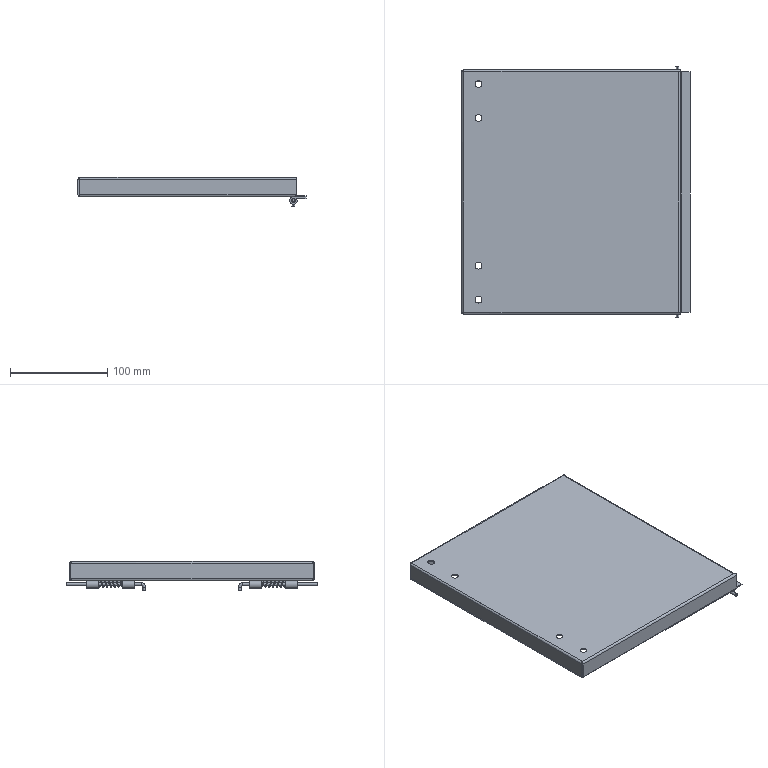Part | 5 solids | 140 faces | box 234.8 x 258.127 x 30 mm | volume 104391 mm3 | plane 74 | cylinder 48 | spline 14 | torus 4 | commonest cylinder face diameters 1.473 x8 3 x8 3.6 x8 3.873 x8 7 x8 7.6 x8